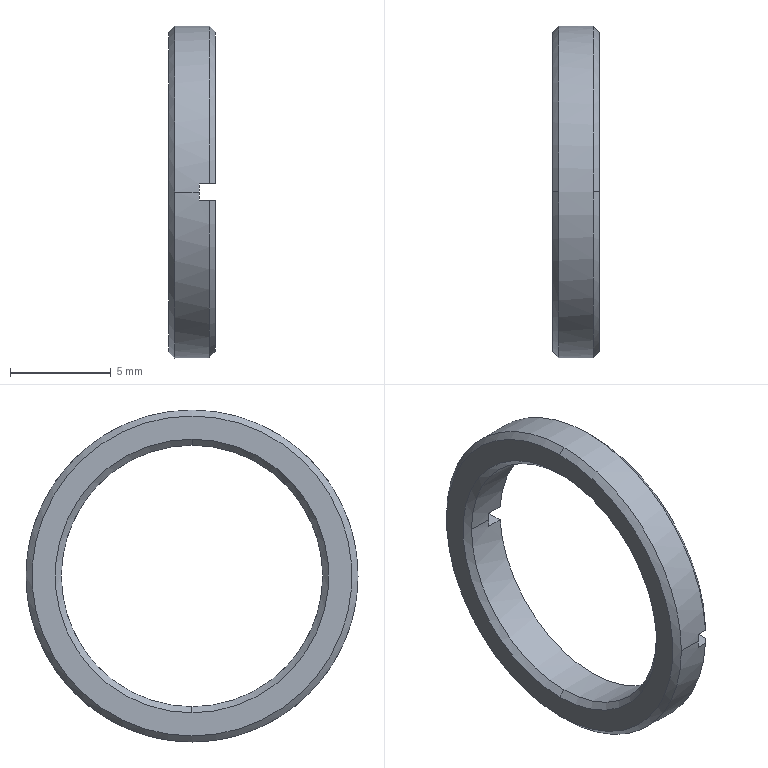Part | STEP file | pressure ring 2.stp.STEP-267.STEP | 1 solid | 20 faces | box 2.3 x 16.5 x 16.5 mm | volume 177.868 mm3 | plane 9 | cone 7 | cylinder 4 | commonest cylinder face diameters 13 x2 16.5 x2
STEP:
#1=CARTESIAN_POINT('',(421.126,0.,-8.25));
#2=VERTEX_POINT('',#1);
#3=CARTESIAN_POINT('',(421.126,8.25,0.));
#4=VERTEX_POINT('',#3);
#5=CARTESIAN_POINT('',(421.126,0.,0.));
#6=DIRECTION('',(1.,0.,0.));
#7=DIRECTION('',(0.,0.,1.));
#8=AXIS2_PLACEMENT_3D('',#5,#6,#7);
#9=CIRCLE('',#8,8.25);
#10=EDGE_CURVE('',#2,#4,#9,.T.);
#11=ORIENTED_EDGE('',*,*,#10,.T.);
#12=CARTESIAN_POINT('',(422.326,8.25,0.));
#13=VERTEX_POINT('',#12);
#14=CARTESIAN_POINT('',(0.,8.25,0.));
#15=DIRECTION('',(1.,0.,0.));
#16=VECTOR('',#15,1000.);
#17=LINE('',#14,#16);
#18=EDGE_CURVE('',#4,#13,#17,.T.);
#19=ORIENTED_EDGE('',*,*,#18,.T.);
#20=CARTESIAN_POINT('',(422.326,8.24,-0.4));
#21=VERTEX_POINT('',#20);
#22=CARTESIAN_POINT('',(422.326,0.,0.));
#23=DIRECTION('',(1.,0.,0.));
#24=DIRECTION('',(0.,0.,1.));
#25=AXIS2_PLACEMENT_3D('',#22,#23,#24);
#26=CIRCLE('',#25,8.25);
#27=EDGE_CURVE('',#21,#13,#26,.T.);
#28=ORIENTED_EDGE('',*,*,#27,.F.);
#29=CARTESIAN_POINT('',(422.826,8.24,-0.4));
#30=VERTEX_POINT('',#29);
#31=CARTESIAN_POINT('',(0.,8.24,-0.4));
#32=DIRECTION('',(1.,0.,0.));
#33=VECTOR('',#32,1000.);
#34=LINE('',#31,#33);
#35=EDGE_CURVE('',#21,#30,#34,.T.);
#36=ORIENTED_EDGE('',*,*,#35,.T.);
#37=CARTESIAN_POINT('',(422.826,-8.24,-0.4));
#38=VERTEX_POINT('',#37);
#39=CARTESIAN_POINT('',(422.826,0.,0.));
#40=DIRECTION('',(-1.,0.,0.));
#41=DIRECTION('',(0.,0.,-1.));
#42=AXIS2_PLACEMENT_3D('',#39,#40,#41);
#43=CIRCLE('',#42,8.25);
#44=EDGE_CURVE('',#30,#38,#43,.T.);
#45=ORIENTED_EDGE('',*,*,#44,.T.);
#46=CARTESIAN_POINT('',(422.326,-8.24,-0.4));
#47=VERTEX_POINT('',#46);
#48=CARTESIAN_POINT('',(0.,-8.24,-0.4));
#49=DIRECTION('',(-1.,0.,0.));
#50=VECTOR('',#49,1000.);
#51=LINE('',#48,#50);
#52=EDGE_CURVE('',#38,#47,#51,.T.);
#53=ORIENTED_EDGE('',*,*,#52,.T.);
#54=CARTESIAN_POINT('',(422.326,-8.25,0.));
#55=VERTEX_POINT('',#54);
#56=CARTESIAN_POINT('',(422.326,0.,0.));
#57=DIRECTION('',(1.,0.,0.));
#58=DIRECTION('',(0.,0.,1.));
#59=AXIS2_PLACEMENT_3D('',#56,#57,#58);
#60=CIRCLE('',#59,8.25);
#61=EDGE_CURVE('',#55,#47,#60,.T.);
#62=ORIENTED_EDGE('',*,*,#61,.F.);
#63=CARTESIAN_POINT('',(421.126,-8.25,0.));
#64=VERTEX_POINT('',#63);
#65=CARTESIAN_POINT('',(0.,-8.25,0.));
#66=DIRECTION('',(1.,0.,0.));
#67=VECTOR('',#66,1000.);
#68=LINE('',#65,#67);
#69=EDGE_CURVE('',#64,#55,#68,.T.);
#70=ORIENTED_EDGE('',*,*,#69,.F.);
#71=CARTESIAN_POINT('',(421.126,0.,0.));
#72=DIRECTION('',(1.,0.,0.));
#73=DIRECTION('',(0.,0.,1.));
#74=AXIS2_PLACEMENT_3D('',#71,#72,#73);
#75=CIRCLE('',#74,8.25);
#76=EDGE_CURVE('',#64,#2,#75,.T.);
#77=ORIENTED_EDGE('',*,*,#76,.T.);
#78=EDGE_LOOP('',(#11,#19,#28,#36,#45,#53,#62,#70,#77));
#79=FACE_OUTER_BOUND('',#78,.T.);
#80=CARTESIAN_POINT('',(0.,0.,0.));
#81=DIRECTION('',(1.,0.,0.));
#82=DIRECTION('',(0.,-1.,0.));
#83=AXIS2_PLACEMENT_3D('',#80,#81,#82);
#84=CYLINDRICAL_SURFACE('',#83,8.25);
#85=ADVANCED_FACE('',(#79),#84,.T.);
#86=CARTESIAN_POINT('',(421.126,0.,6.5));
#87=VERTEX_POINT('',#86);
#88=CARTESIAN_POINT('',(421.126,6.5,0.));
#89=VERTEX_POINT('',#88);
#90=CARTESIAN_POINT('',(421.126,0.,0.));
#91=DIRECTION('',(-1.,0.,0.));
#92=DIRECTION('',(0.,0.,1.));
#93=AXIS2_PLACEMENT_3D('',#90,#91,#92);
#94=CIRCLE('',#93,6.5);
#95=EDGE_CURVE('',#87,#89,#94,.T.);
#96=ORIENTED_EDGE('',*,*,#95,.T.);
#97=CARTESIAN_POINT('',(422.326,6.5,0.));
#98=VERTEX_POINT('',#97);
#99=CARTESIAN_POINT('',(0.,6.5,0.));
#100=DIRECTION('',(1.,0.,0.));
#101=VECTOR('',#100,1000.);
#102=LINE('',#99,#101);
#103=EDGE_CURVE('',#89,#98,#102,.T.);
#104=ORIENTED_EDGE('',*,*,#103,.T.);
#105=CARTESIAN_POINT('',(422.326,6.488,0.4));
#106=VERTEX_POINT('',#105);
#107=CARTESIAN_POINT('',(422.326,0.,0.));
#108=DIRECTION('',(-1.,0.,0.));
#109=DIRECTION('',(0.,0.,1.));
#110=AXIS2_PLACEMENT_3D('',#107,#108,#109);
#111=CIRCLE('',#110,6.5);
#112=EDGE_CURVE('',#106,#98,#111,.T.);
#113=ORIENTED_EDGE('',*,*,#112,.F.);
#114=CARTESIAN_POINT('',(423.126,6.488,0.4));
#115=VERTEX_POINT('',#114);
#116=CARTESIAN_POINT('',(0.,6.488,0.4));
#117=DIRECTION('',(1.,0.,0.));
#118=VECTOR('',#117,1000.);
#119=LINE('',#116,#118);
#120=EDGE_CURVE('',#106,#115,#119,.T.);
#121=ORIENTED_EDGE('',*,*,#120,.T.);
#122=CARTESIAN_POINT('',(423.126,-6.488,0.4));
#123=VERTEX_POINT('',#122);
#124=CARTESIAN_POINT('',(423.126,0.,0.));
#125=DIRECTION('',(1.,0.,0.));
#126=DIRECTION('',(0.,-1.,0.));
#127=AXIS2_PLACEMENT_3D('',#124,#125,#126);
#128=CIRCLE('',#127,6.5);
#129=EDGE_CURVE('',#115,#123,#128,.T.);
#130=ORIENTED_EDGE('',*,*,#129,.T.);
#131=CARTESIAN_POINT('',(422.326,-6.488,0.4));
#132=VERTEX_POINT('',#131);
#133=CARTESIAN_POINT('',(0.,-6.488,0.4));
#134=DIRECTION('',(-1.,0.,0.));
#135=VECTOR('',#134,1000.);
#136=LINE('',#133,#135);
#137=EDGE_CURVE('',#123,#132,#136,.T.);
#138=ORIENTED_EDGE('',*,*,#137,.T.);
#139=CARTESIAN_POINT('',(422.326,-6.5,0.));
#140=VERTEX_POINT('',#139);
#141=CARTESIAN_POINT('',(422.326,0.,0.));
#142=DIRECTION('',(-1.,0.,0.));
#143=DIRECTION('',(0.,0.,1.));
#144=AXIS2_PLACEMENT_3D('',#141,#142,#143);
#145=CIRCLE('',#144,6.5);
#146=EDGE_CURVE('',#140,#132,#145,.T.);
#147=ORIENTED_EDGE('',*,*,#146,.F.);
#148=CARTESIAN_POINT('',(421.126,-6.5,0.));
#149=VERTEX_POINT('',#148);
#150=CARTESIAN_POINT('',(0.,-6.5,0.));
#151=DIRECTION('',(1.,0.,0.));
#152=VECTOR('',#151,1000.);
#153=LINE('',#150,#152);
#154=EDGE_CURVE('',#149,#140,#153,.T.);
#155=ORIENTED_EDGE('',*,*,#154,.F.);
#156=CARTESIAN_POINT('',(421.126,0.,0.));
#157=DIRECTION('',(-1.,0.,0.));
#158=DIRECTION('',(0.,0.,1.));
#159=AXIS2_PLACEMENT_3D('',#156,#157,#158);
#160=CIRCLE('',#159,6.5);
#161=EDGE_CURVE('',#149,#87,#160,.T.);
#162=ORIENTED_EDGE('',*,*,#161,.T.);
#163=EDGE_LOOP('',(#96,#104,#113,#121,#130,#138,#147,#155,#162));
#164=FACE_OUTER_BOUND('',#163,.T.);
#165=CARTESIAN_POINT('',(0.,0.,0.));
#166=DIRECTION('',(1.,0.,0.));
#167=DIRECTION('',(0.,-1.,0.));
#168=AXIS2_PLACEMENT_3D('',#165,#166,#167);
#169=CYLINDRICAL_SURFACE('',#168,6.5);
#170=ADVANCED_FACE('',(#164),#169,.F.);
#171=CARTESIAN_POINT('',(421.126,0.,-6.5));
#172=VERTEX_POINT('',#171);
#173=CARTESIAN_POINT('',(421.126,0.,0.));
#174=DIRECTION('',(-1.,0.,0.));
#175=DIRECTION('',(0.,0.,1.));
#176=AXIS2_PLACEMENT_3D('',#173,#174,#175);
#177=CIRCLE('',#176,6.5);
#178=EDGE_CURVE('',#172,#149,#177,.T.);
#179=ORIENTED_EDGE('',*,*,#178,.F.);
#180=CARTESIAN_POINT('',(420.826,0.,-6.8));
#181=VERTEX_POINT('',#180);
#182=CARTESIAN_POINT('',(420.826,0.,-6.8));
#183=DIRECTION('',(-0.7071,0.,-0.7071));
#184=VECTOR('',#183,1000.);
#185=LINE('',#182,#184);
#186=EDGE_CURVE('',#172,#181,#185,.T.);
#187=ORIENTED_EDGE('',*,*,#186,.T.);
#188=CARTESIAN_POINT('',(420.826,0.,6.8));
#189=VERTEX_POINT('',#188);
#190=CARTESIAN_POINT('',(420.826,0.,0.));
#191=DIRECTION('',(1.,0.,0.));
#192=DIRECTION('',(0.,0.,1.));
#193=AXIS2_PLACEMENT_3D('',#190,#191,#192);
#194=CIRCLE('',#193,6.8);
#195=EDGE_CURVE('',#189,#181,#194,.T.);
#196=ORIENTED_EDGE('',*,*,#195,.F.);
#197=CARTESIAN_POINT('',(420.826,0.,6.8));
#198=DIRECTION('',(-0.7071,0.,0.7071));
#199=VECTOR('',#198,1000.);
#200=LINE('',#197,#199);
#201=EDGE_CURVE('',#87,#189,#200,.T.);
#202=ORIENTED_EDGE('',*,*,#201,.F.);
#203=ORIENTED_EDGE('',*,*,#161,.F.);
#204=EDGE_LOOP('',(#179,#187,#196,#202,#203));
#205=FACE_OUTER_BOUND('',#204,.T.);
#206=CARTESIAN_POINT('',(420.826,0.,0.));
#207=DIRECTION('',(-1.,0.,0.));
#208=DIRECTION('',(0.,0.,1.));
#209=AXIS2_PLACEMENT_3D('',#206,#207,#208);
#210=CONICAL_SURFACE('',#209,6.8,0.7854);
#211=ADVANCED_FACE('',(#205),#210,.F.);
#212=CARTESIAN_POINT('',(423.126,0.,7.95));
#213=VERTEX_POINT('',#212);
#214=CARTESIAN_POINT('',(423.126,-7.94,0.4));
#215=VERTEX_POINT('',#214);
#216=CARTESIAN_POINT('',(423.126,0.,0.));
#217=DIRECTION('',(1.,0.,0.));
#218=DIRECTION('',(0.,0.,-1.));
#219=AXIS2_PLACEMENT_3D('',#216,#217,#218);
#220=CIRCLE('',#219,7.95);
#221=EDGE_CURVE('',#213,#215,#220,.T.);
#222=ORIENTED_EDGE('',*,*,#221,.F.);
#223=CARTESIAN_POINT('',(422.826,0.,8.25));
#224=VERTEX_POINT('',#223);
#225=CARTESIAN_POINT('',(423.126,0.,7.95));
#226=DIRECTION('',(-0.7071,0.,0.7071));
#227=VECTOR('',#226,1000.);
#228=LINE('',#225,#227);
#229=EDGE_CURVE('',#213,#224,#228,.T.);
#230=ORIENTED_EDGE('',*,*,#229,.T.);
#231=CARTESIAN_POINT('',(422.826,-8.24,0.4));
#232=VERTEX_POINT('',#231);
#233=CARTESIAN_POINT('',(422.826,0.,0.));
#234=DIRECTION('',(-1.,0.,0.));
#235=DIRECTION('',(0.,0.,-1.));
#236=AXIS2_PLACEMENT_3D('',#233,#234,#235);
#237=CIRCLE('',#236,8.25);
#238=EDGE_CURVE('',#232,#224,#237,.T.);
#239=ORIENTED_EDGE('',*,*,#238,.F.);
#240=CARTESIAN_POINT('',(423.126,-7.94,0.4));
#241=CARTESIAN_POINT('',(423.026,-8.04,0.4));
#242=CARTESIAN_POINT('',(422.926,-8.14,0.4));
#243=CARTESIAN_POINT('',(422.826,-8.24,0.4));
#244=B_SPLINE_CURVE_WITH_KNOTS('',3,(#240,#241,#242,#243),.UNSPECIFIED.,.F.,.F.,(4,4),(0.,0.0004245),.UNSPECIFIED.);
#245=EDGE_CURVE('',#215,#232,#244,.T.);
#246=ORIENTED_EDGE('',*,*,#245,.F.);
#247=EDGE_LOOP('',(#222,#230,#239,#246));
#248=FACE_OUTER_BOUND('',#247,.T.);
#249=CARTESIAN_POINT('',(423.126,0.,0.));
#250=DIRECTION('',(-1.,0.,0.));
#251=DIRECTION('',(0.,0.,1.));
#252=AXIS2_PLACEMENT_3D('',#249,#250,#251);
#253=CONICAL_SURFACE('',#252,7.95,0.7854);
#254=ADVANCED_FACE('',(#248),#253,.T.);
#255=CARTESIAN_POINT('',(420.826,0.,7.95));
#256=VERTEX_POINT('',#255);
#257=CARTESIAN_POINT('',(420.826,0.,-7.95));
#258=VERTEX_POINT('',#257);
#259=CARTESIAN_POINT('',(420.826,0.,0.));
#260=DIRECTION('',(-1.,0.,0.));
#261=DIRECTION('',(0.,0.,1.));
#262=AXIS2_PLACEMENT_3D('',#259,#260,#261);
#263=CIRCLE('',#262,7.95);
#264=EDGE_CURVE('',#256,#258,#263,.T.);
#265=ORIENTED_EDGE('',*,*,#264,.F.);
#266=CARTESIAN_POINT('',(421.126,0.,8.25));
#267=VERTEX_POINT('',#266);
#268=CARTESIAN_POINT('',(421.126,0.,8.25));
#269=DIRECTION('',(0.7071,0.,0.7071));
#270=VECTOR('',#269,1000.);
#271=LINE('',#268,#270);
#272=EDGE_CURVE('',#256,#267,#271,.T.);
#273=ORIENTED_EDGE('',*,*,#272,.T.);
#274=CARTESIAN_POINT('',(421.126,0.,0.));
#275=DIRECTION('',(1.,0.,0.));
#276=DIRECTION('',(0.,0.,1.));
#277=AXIS2_PLACEMENT_3D('',#274,#275,#276);
#278=CIRCLE('',#277,8.25);
#279=EDGE_CURVE('',#4,#267,#278,.T.);
#280=ORIENTED_EDGE('',*,*,#279,.F.);
#281=ORIENTED_EDGE('',*,*,#10,.F.);
#282=CARTESIAN_POINT('',(421.126,0.,-8.25));
#283=DIRECTION('',(0.7071,0.,-0.7071));
#284=VECTOR('',#283,1000.);
#285=LINE('',#282,#284);
#286=EDGE_CURVE('',#258,#2,#285,.T.);
#287=ORIENTED_EDGE('',*,*,#286,.F.);
#288=EDGE_LOOP('',(#265,#273,#280,#281,#287));
#289=FACE_OUTER_BOUND('',#288,.T.);
#290=CARTESIAN_POINT('',(421.126,0.,0.));
#291=DIRECTION('',(1.,0.,0.));
#292=DIRECTION('',(0.,0.,-1.));
#293=AXIS2_PLACEMENT_3D('',#290,#291,#292);
#294=CONICAL_SURFACE('',#293,8.25,0.7854);
#295=ADVANCED_FACE('',(#289),#294,.T.);
#296=ORIENTED_EDGE('',*,*,#272,.F.);
#297=CARTESIAN_POINT('',(420.826,0.,0.));
#298=DIRECTION('',(-1.,0.,0.));
#299=DIRECTION('',(0.,0.,1.));
#300=AXIS2_PLACEMENT_3D('',#297,#298,#299);
#301=CIRCLE('',#300,7.95);
#302=EDGE_CURVE('',#258,#256,#301,.T.);
#303=ORIENTED_EDGE('',*,*,#302,.F.);
#304=ORIENTED_EDGE('',*,*,#286,.T.);
#305=ORIENTED_EDGE('',*,*,#76,.F.);
#306=CARTESIAN_POINT('',(421.126,0.,0.));
#307=DIRECTION('',(1.,0.,0.));
#308=DIRECTION('',(0.,0.,1.));
#309=AXIS2_PLACEMENT_3D('',#306,#307,#308);
#310=CIRCLE('',#309,8.25);
#311=EDGE_CURVE('',#267,#64,#310,.T.);
#312=ORIENTED_EDGE('',*,*,#311,.F.);
#313=EDGE_LOOP('',(#296,#303,#304,#305,#312));
#314=FACE_OUTER_BOUND('',#313,.T.);
#315=CARTESIAN_POINT('',(421.126,0.,0.));
#316=DIRECTION('',(1.,0.,0.));
#317=DIRECTION('',(0.,0.,-1.));
#318=AXIS2_PLACEMENT_3D('',#315,#316,#317);
#319=CONICAL_SURFACE('',#318,8.25,0.7854);
#320=ADVANCED_FACE('',(#314),#319,.T.);
#321=ORIENTED_EDGE('',*,*,#229,.F.);
#322=CARTESIAN_POINT('',(423.126,7.94,0.4));
#323=VERTEX_POINT('',#322);
#324=CARTESIAN_POINT('',(423.126,0.,0.));
#325=DIRECTION('',(1.,0.,0.));
#326=DIRECTION('',(0.,0.,-1.));
#327=AXIS2_PLACEMENT_3D('',#324,#325,#326);
#328=CIRCLE('',#327,7.95);
#329=EDGE_CURVE('',#323,#213,#328,.T.);
#330=ORIENTED_EDGE('',*,*,#329,.F.);
#331=CARTESIAN_POINT('',(422.826,8.24,0.4));
#332=VERTEX_POINT('',#331);
#333=CARTESIAN_POINT('',(422.826,8.24,0.4));
#334=CARTESIAN_POINT('',(422.926,8.14,0.4));
#335=CARTESIAN_POINT('',(423.026,8.04,0.4));
#336=CARTESIAN_POINT('',(423.126,7.94,0.4));
#337=B_SPLINE_CURVE_WITH_KNOTS('',3,(#333,#334,#335,#336),.UNSPECIFIED.,.F.,.F.,(4,4),(0.,0.0004245),.UNSPECIFIED.);
#338=EDGE_CURVE('',#332,#323,#337,.T.);
#339=ORIENTED_EDGE('',*,*,#338,.F.);
#340=CARTESIAN_POINT('',(422.826,0.,0.));
#341=DIRECTION('',(-1.,0.,0.));
#342=DIRECTION('',(0.,0.,-1.));
#343=AXIS2_PLACEMENT_3D('',#340,#341,#342);
#344=CIRCLE('',#343,8.25);
#345=EDGE_CURVE('',#224,#332,#344,.T.);
#346=ORIENTED_EDGE('',*,*,#345,.F.);
#347=EDGE_LOOP('',(#321,#330,#339,#346));
#348=FACE_OUTER_BOUND('',#347,.T.);
#349=CARTESIAN_POINT('',(423.126,0.,0.));
#350=DIRECTION('',(-1.,0.,0.));
#351=DIRECTION('',(0.,0.,1.));
#352=AXIS2_PLACEMENT_3D('',#349,#350,#351);
#353=CONICAL_SURFACE('',#352,7.95,0.7854);
#354=ADVANCED_FACE('',(#348),#353,.T.);
#355=CARTESIAN_POINT('',(423.126,10.,0.4));
#356=DIRECTION('',(0.,-1.,0.));
#357=VECTOR('',#356,1000.);
#358=LINE('',#355,#357);
#359=EDGE_CURVE('',#323,#115,#358,.T.);
#360=ORIENTED_EDGE('',*,*,#359,.F.);
#361=ORIENTED_EDGE('',*,*,#329,.T.);
#362=ORIENTED_EDGE('',*,*,#221,.T.);
#363=CARTESIAN_POINT('',(423.126,10.,0.4));
#364=DIRECTION('',(0.,-1.,0.));
#365=VECTOR('',#364,1000.);
#366=LINE('',#363,#365);
#367=EDGE_CURVE('',#123,#215,#366,.T.);
#368=ORIENTED_EDGE('',*,*,#367,.F.);
#369=ORIENTED_EDGE('',*,*,#129,.F.);
#370=EDGE_LOOP('',(#360,#361,#362,#368,#369));
#371=FACE_OUTER_BOUND('',#370,.T.);
#372=CARTESIAN_POINT('',(423.126,6.5,0.));
#373=DIRECTION('',(1.,0.,0.));
#374=DIRECTION('',(0.,1.,0.));
#375=AXIS2_PLACEMENT_3D('',#372,#373,#374);
#376=PLANE('',#375);
#377=ADVANCED_FACE('',(#371),#376,.T.);
#378=ORIENTED_EDGE('',*,*,#52,.F.);
#379=CARTESIAN_POINT('',(423.126,-7.94,-0.4));
#380=VERTEX_POINT('',#379);
#381=CARTESIAN_POINT('',(422.826,-8.24,-0.4));
#382=CARTESIAN_POINT('',(422.926,-8.14,-0.4));
#383=CARTESIAN_POINT('',(423.026,-8.04,-0.4));
#384=CARTESIAN_POINT('',(423.126,-7.94,-0.4));
#385=B_SPLINE_CURVE_WITH_KNOTS('',3,(#381,#382,#383,#384),.UNSPECIFIED.,.F.,.F.,(4,4),(0.,0.0004245),.UNSPECIFIED.);
#386=EDGE_CURVE('',#38,#380,#385,.T.);
#387=ORIENTED_EDGE('',*,*,#386,.T.);
#388=CARTESIAN_POINT('',(423.126,-6.488,-0.4));
#389=VERTEX_POINT('',#388);
#390=CARTESIAN_POINT('',(423.126,-10.,-0.4));
#391=DIRECTION('',(0.,1.,0.));
#392=VECTOR('',#391,1000.);
#393=LINE('',#390,#392);
#394=EDGE_CURVE('',#380,#389,#393,.T.);
#395=ORIENTED_EDGE('',*,*,#394,.T.);
#396=CARTESIAN_POINT('',(422.326,-6.488,-0.4));
#397=VERTEX_POINT('',#396);
#398=CARTESIAN_POINT('',(0.,-6.488,-0.4));
#399=DIRECTION('',(1.,0.,0.));
#400=VECTOR('',#399,1000.);
#401=LINE('',#398,#400);
#402=EDGE_CURVE('',#397,#389,#401,.T.);
#403=ORIENTED_EDGE('',*,*,#402,.F.);
#404=CARTESIAN_POINT('',(422.326,-10.,-0.4));
#405=DIRECTION('',(0.,1.,0.));
#406=VECTOR('',#405,1000.);
#407=LINE('',#404,#406);
#408=EDGE_CURVE('',#47,#397,#407,.T.);
#409=ORIENTED_EDGE('',*,*,#408,.F.);
#410=EDGE_LOOP('',(#378,#387,#395,#403,#409));
#411=FACE_OUTER_BOUND('',#410,.T.);
#412=CARTESIAN_POINT('',(422.326,-10.,-0.4));
#413=DIRECTION('',(0.,0.,1.));
#414=DIRECTION('',(0.,-1.,0.));
#415=AXIS2_PLACEMENT_3D('',#412,#413,#414);
#416=PLANE('',#415);
#417=ADVANCED_FACE('',(#411),#416,.T.);
#418=CARTESIAN_POINT('',(422.326,8.24,0.4));
#419=VERTEX_POINT('',#418);
#420=CARTESIAN_POINT('',(0.,8.24,0.4));
#421=DIRECTION('',(-1.,0.,0.));
#422=VECTOR('',#421,1000.);
#423=LINE('',#420,#422);
#424=EDGE_CURVE('',#332,#419,#423,.T.);
#425=ORIENTED_EDGE('',*,*,#424,.F.);
#426=ORIENTED_EDGE('',*,*,#338,.T.);
#427=ORIENTED_EDGE('',*,*,#359,.T.);
#428=ORIENTED_EDGE('',*,*,#120,.F.);
#429=CARTESIAN_POINT('',(422.326,10.,0.4));
#430=DIRECTION('',(0.,-1.,0.));
#431=VECTOR('',#430,1000.);
#432=LINE('',#429,#431);
#433=EDGE_CURVE('',#419,#106,#432,.T.);
#434=ORIENTED_EDGE('',*,*,#433,.F.);
#435=EDGE_LOOP('',(#425,#426,#427,#428,#434));
#436=FACE_OUTER_BOUND('',#435,.T.);
#437=CARTESIAN_POINT('',(422.326,10.,0.4));
#438=DIRECTION('',(0.,0.,-1.));
#439=DIRECTION('',(-1.,0.,0.));
#440=AXIS2_PLACEMENT_3D('',#437,#438,#439);
#441=PLANE('',#440);
#442=ADVANCED_FACE('',(#436),#441,.T.);
#443=CARTESIAN_POINT('',(423.126,6.488,-0.4));
#444=VERTEX_POINT('',#443);
#445=CARTESIAN_POINT('',(423.126,7.94,-0.4));
#446=VERTEX_POINT('',#445);
#447=CARTESIAN_POINT('',(423.126,-10.,-0.4));
#448=DIRECTION('',(0.,1.,0.));
#449=VECTOR('',#448,1000.);
#450=LINE('',#447,#449);
#451=EDGE_CURVE('',#444,#446,#450,.T.);
#452=ORIENTED_EDGE('',*,*,#451,.T.);
#453=CARTESIAN_POINT('',(423.126,7.94,-0.4));
#454=CARTESIAN_POINT('',(423.026,8.04,-0.4));
#455=CARTESIAN_POINT('',(422.926,8.14,-0.4));
#456=CARTESIAN_POINT('',(422.826,8.24,-0.4));
#457=B_SPLINE_CURVE_WITH_KNOTS('',3,(#453,#454,#455,#456),.UNSPECIFIED.,.F.,.F.,(4,4),(0.,0.0004245),.UNSPECIFIED.);
#458=EDGE_CURVE('',#446,#30,#457,.T.);
#459=ORIENTED_EDGE('',*,*,#458,.T.);
#460=ORIENTED_EDGE('',*,*,#35,.F.);
#461=CARTESIAN_POINT('',(422.326,6.488,-0.4));
#462=VERTEX_POINT('',#461);
#463=CARTESIAN_POINT('',(422.326,-10.,-0.4));
#464=DIRECTION('',(0.,1.,0.));
#465=VECTOR('',#464,1000.);
#466=LINE('',#463,#465);
#467=EDGE_CURVE('',#462,#21,#466,.T.);
#468=ORIENTED_EDGE('',*,*,#467,.F.);
#469=CARTESIAN_POINT('',(0.,6.488,-0.4));
#470=DIRECTION('',(-1.,0.,0.));
#471=VECTOR('',#470,1000.);
#472=LINE('',#469,#471);
#473=EDGE_CURVE('',#444,#462,#472,.T.);
#474=ORIENTED_EDGE('',*,*,#473,.F.);
#475=EDGE_LOOP('',(#452,#459,#460,#468,#474));
#476=FACE_OUTER_BOUND('',#475,.T.);
#477=CARTESIAN_POINT('',(422.326,-10.,-0.4));
#478=DIRECTION('',(0.,0.,1.));
#479=DIRECTION('',(0.,-1.,0.));
#480=AXIS2_PLACEMENT_3D('',#477,#478,#479);
#481=PLANE('',#480);
#482=ADVANCED_FACE('',(#476),#481,.T.);
#483=ORIENTED_EDGE('',*,*,#112,.T.);
#484=CARTESIAN_POINT('',(422.326,0.,0.));
#485=DIRECTION('',(-1.,0.,0.));
#486=DIRECTION('',(0.,0.,1.));
#487=AXIS2_PLACEMENT_3D('',#484,#485,#486);
#488=CIRCLE('',#487,6.5);
#489=EDGE_CURVE('',#98,#462,#488,.T.);
#490=ORIENTED_EDGE('',*,*,#489,.T.);
#491=ORIENTED_EDGE('',*,*,#467,.T.);
#492=ORIENTED_EDGE('',*,*,#27,.T.);
#493=CARTESIAN_POINT('',(422.326,0.,0.));
#494=DIRECTION('',(1.,0.,0.));
#495=DIRECTION('',(0.,0.,1.));
#496=AXIS2_PLACEMENT_3D('',#493,#494,#495);
#497=CIRCLE('',#496,8.25);
#498=EDGE_CURVE('',#13,#419,#497,.T.);
#499=ORIENTED_EDGE('',*,*,#498,.T.);
#500=ORIENTED_EDGE('',*,*,#433,.T.);
#501=EDGE_LOOP('',(#483,#490,#491,#492,#499,#500));
#502=FACE_OUTER_BOUND('',#501,.T.);
#503=CARTESIAN_POINT('',(422.326,10.,0.4));
#504=DIRECTION('',(-1.,0.,0.));
#505=DIRECTION('',(0.,0.,1.));
#506=AXIS2_PLACEMENT_3D('',#503,#504,#505);
#507=PLANE('',#506);
#508=ADVANCED_FACE('',(#502),#507,.F.);
#509=CARTESIAN_POINT('',(422.326,0.,0.));
#510=DIRECTION('',(-1.,0.,0.));
#511=DIRECTION('',(0.,0.,1.));
#512=AXIS2_PLACEMENT_3D('',#509,#510,#511);
#513=CIRCLE('',#512,6.5);
#514=EDGE_CURVE('',#397,#140,#513,.T.);
#515=ORIENTED_EDGE('',*,*,#514,.T.);
#516=ORIENTED_EDGE('',*,*,#146,.T.);
#517=CARTESIAN_POINT('',(422.326,-8.24,0.4));
#518=VERTEX_POINT('',#517);
#519=CARTESIAN_POINT('',(422.326,10.,0.4));
#520=DIRECTION('',(0.,-1.,0.));
#521=VECTOR('',#520,1000.);
#522=LINE('',#519,#521);
#523=EDGE_CURVE('',#132,#518,#522,.T.);
#524=ORIENTED_EDGE('',*,*,#523,.T.);
#525=CARTESIAN_POINT('',(422.326,0.,0.));
#526=DIRECTION('',(1.,0.,0.));
#527=DIRECTION('',(0.,0.,1.));
#528=AXIS2_PLACEMENT_3D('',#525,#526,#527);
#529=CIRCLE('',#528,8.25);
#530=EDGE_CURVE('',#518,#55,#529,.T.);
#531=ORIENTED_EDGE('',*,*,#530,.T.);
#532=ORIENTED_EDGE('',*,*,#61,.T.);
#533=ORIENTED_EDGE('',*,*,#408,.T.);
#534=EDGE_LOOP('',(#515,#516,#524,#531,#532,#533));
#535=FACE_OUTER_BOUND('',#534,.T.);
#536=CARTESIAN_POINT('',(422.326,10.,0.4));
#537=DIRECTION('',(-1.,0.,0.));
#538=DIRECTION('',(0.,0.,1.));
#539=AXIS2_PLACEMENT_3D('',#536,#537,#538);
#540=PLANE('',#539);
#541=ADVANCED_FACE('',(#535),#540,.F.);
#542=ORIENTED_EDGE('',*,*,#186,.F.);
#543=CARTESIAN_POINT('',(421.126,0.,0.));
#544=DIRECTION('',(-1.,0.,0.));
#545=DIRECTION('',(0.,0.,1.));
#546=AXIS2_PLACEMENT_3D('',#543,#544,#545);
#547=CIRCLE('',#546,6.5);
#548=EDGE_CURVE('',#89,#172,#547,.T.);
#549=ORIENTED_EDGE('',*,*,#548,.F.);
#550=ORIENTED_EDGE('',*,*,#95,.F.);
#551=ORIENTED_EDGE('',*,*,#201,.T.);
#552=CARTESIAN_POINT('',(420.826,0.,0.));
#553=DIRECTION('',(1.,0.,0.));
#554=DIRECTION('',(0.,0.,1.));
#555=AXIS2_PLACEMENT_3D('',#552,#553,#554);
#556=CIRCLE('',#555,6.8);
#557=EDGE_CURVE('',#181,#189,#556,.T.);
#558=ORIENTED_EDGE('',*,*,#557,.F.);
#559=EDGE_LOOP('',(#542,#549,#550,#551,#558));
#560=FACE_OUTER_BOUND('',#559,.T.);
#561=CARTESIAN_POINT('',(420.826,0.,0.));
#562=DIRECTION('',(-1.,0.,0.));
#563=DIRECTION('',(0.,0.,1.));
#564=AXIS2_PLACEMENT_3D('',#561,#562,#563);
#565=CONICAL_SURFACE('',#564,6.8,0.7854);
#566=ADVANCED_FACE('',(#560),#565,.F.);
#567=ORIENTED_EDGE('',*,*,#195,.T.);
#568=ORIENTED_EDGE('',*,*,#557,.T.);
#569=EDGE_LOOP('',(#567,#568));
#570=FACE_BOUND('',#569,.T.);
#571=ORIENTED_EDGE('',*,*,#302,.T.);
#572=ORIENTED_EDGE('',*,*,#264,.T.);
#573=EDGE_LOOP('',(#571,#572));
#574=FACE_OUTER_BOUND('',#573,.T.);
#575=CARTESIAN_POINT('',(420.826,8.25,0.));
#576=DIRECTION('',(-1.,0.,0.));
#577=DIRECTION('',(0.,0.,1.));
#578=AXIS2_PLACEMENT_3D('',#575,#576,#577);
#579=PLANE('',#578);
#580=ADVANCED_FACE('',(#570,#574),#579,.T.);
#581=ORIENTED_EDGE('',*,*,#103,.F.);
#582=ORIENTED_EDGE('',*,*,#548,.T.);
#583=ORIENTED_EDGE('',*,*,#178,.T.);
#584=ORIENTED_EDGE('',*,*,#154,.T.);
#585=ORIENTED_EDGE('',*,*,#514,.F.);
#586=ORIENTED_EDGE('',*,*,#402,.T.);
#587=CARTESIAN_POINT('',(423.126,0.,0.));
#588=DIRECTION('',(1.,0.,0.));
#589=DIRECTION('',(0.,-1.,0.));
#590=AXIS2_PLACEMENT_3D('',#587,#588,#589);
#591=CIRCLE('',#590,6.5);
#592=EDGE_CURVE('',#389,#444,#591,.T.);
#593=ORIENTED_EDGE('',*,*,#592,.T.);
#594=ORIENTED_EDGE('',*,*,#473,.T.);
#595=ORIENTED_EDGE('',*,*,#489,.F.);
#596=EDGE_LOOP('',(#581,#582,#583,#584,#585,#586,#593,#594,#595));
#597=FACE_OUTER_BOUND('',#596,.T.);
#598=CARTESIAN_POINT('',(0.,0.,0.));
#599=DIRECTION('',(1.,0.,0.));
#600=DIRECTION('',(0.,-1.,0.));
#601=AXIS2_PLACEMENT_3D('',#598,#599,#600);
#602=CYLINDRICAL_SURFACE('',#601,6.5);
#603=ADVANCED_FACE('',(#597),#602,.F.);
#604=ORIENTED_EDGE('',*,*,#394,.F.);
#605=CARTESIAN_POINT('',(423.126,0.,0.));
#606=DIRECTION('',(1.,0.,0.));
#607=DIRECTION('',(0.,0.,-1.));
#608=AXIS2_PLACEMENT_3D('',#605,#606,#607);
#609=CIRCLE('',#608,7.95);
#610=EDGE_CURVE('',#380,#446,#609,.T.);
#611=ORIENTED_EDGE('',*,*,#610,.T.);
#612=ORIENTED_EDGE('',*,*,#451,.F.);
#613=ORIENTED_EDGE('',*,*,#592,.F.);
#614=EDGE_LOOP('',(#604,#611,#612,#613));
#615=FACE_OUTER_BOUND('',#614,.T.);
#616=CARTESIAN_POINT('',(423.126,6.5,0.));
#617=DIRECTION('',(1.,0.,0.));
#618=DIRECTION('',(0.,1.,0.));
#619=AXIS2_PLACEMENT_3D('',#616,#617,#618);
#620=PLANE('',#619);
#621=ADVANCED_FACE('',(#615),#620,.T.);
#622=ORIENTED_EDGE('',*,*,#18,.F.);
#623=ORIENTED_EDGE('',*,*,#279,.T.);
#624=ORIENTED_EDGE('',*,*,#311,.T.);
#625=ORIENTED_EDGE('',*,*,#69,.T.);
#626=ORIENTED_EDGE('',*,*,#530,.F.);
#627=CARTESIAN_POINT('',(0.,-8.24,0.4));
#628=DIRECTION('',(1.,0.,0.));
#629=VECTOR('',#628,1000.);
#630=LINE('',#627,#629);
#631=EDGE_CURVE('',#518,#232,#630,.T.);
#632=ORIENTED_EDGE('',*,*,#631,.T.);
#633=ORIENTED_EDGE('',*,*,#238,.T.);
#634=ORIENTED_EDGE('',*,*,#345,.T.);
#635=ORIENTED_EDGE('',*,*,#424,.T.);
#636=ORIENTED_EDGE('',*,*,#498,.F.);
#637=EDGE_LOOP('',(#622,#623,#624,#625,#626,#632,#633,#634,#635,#636));
#638=FACE_OUTER_BOUND('',#637,.T.);
#639=CARTESIAN_POINT('',(0.,0.,0.));
#640=DIRECTION('',(1.,0.,0.));
#641=DIRECTION('',(0.,-1.,0.));
#642=AXIS2_PLACEMENT_3D('',#639,#640,#641);
#643=CYLINDRICAL_SURFACE('',#642,8.25);
#644=ADVANCED_FACE('',(#638),#643,.T.);
#645=ORIENTED_EDGE('',*,*,#367,.T.);
#646=ORIENTED_EDGE('',*,*,#245,.T.);
#647=ORIENTED_EDGE('',*,*,#631,.F.);
#648=ORIENTED_EDGE('',*,*,#523,.F.);
#649=ORIENTED_EDGE('',*,*,#137,.F.);
#650=EDGE_LOOP('',(#645,#646,#647,#648,#649));
#651=FACE_OUTER_BOUND('',#650,.T.);
#652=CARTESIAN_POINT('',(422.326,10.,0.4));
#653=DIRECTION('',(0.,0.,-1.));
#654=DIRECTION('',(-1.,0.,0.));
#655=AXIS2_PLACEMENT_3D('',#652,#653,#654);
#656=PLANE('',#655);
#657=ADVANCED_FACE('',(#651),#656,.T.);
#658=ORIENTED_EDGE('',*,*,#386,.F.);
#659=ORIENTED_EDGE('',*,*,#44,.F.);
#660=ORIENTED_EDGE('',*,*,#458,.F.);
#661=ORIENTED_EDGE('',*,*,#610,.F.);
#662=EDGE_LOOP('',(#658,#659,#660,#661));
#663=FACE_OUTER_BOUND('',#662,.T.);
#664=CARTESIAN_POINT('',(423.126,0.,0.));
#665=DIRECTION('',(-1.,0.,0.));
#666=DIRECTION('',(0.,0.,1.));
#667=AXIS2_PLACEMENT_3D('',#664,#665,#666);
#668=CONICAL_SURFACE('',#667,7.95,0.7854);
#669=ADVANCED_FACE('',(#663),#668,.T.);
#670=CLOSED_SHELL('',(#85,#170,#211,#254,#295,#320,#354,#377,#417,#442,#482,#508,#541,#566,#580,#603,#621,#644,#657,#669));
#671=MANIFOLD_SOLID_BREP('',#670);
#672=CARTESIAN_POINT('',(0.,0.,0.));
#673=DIRECTION('',(0.,0.,1.));
#674=DIRECTION('',(1.,0.,0.));
#675=AXIS2_PLACEMENT_3D('',#672,#673,#674);
#676=(LENGTH_UNIT()NAMED_UNIT(*)SI_UNIT(.MILLI.,.METRE.));
#677=UNCERTAINTY_MEASURE_WITH_UNIT(LENGTH_MEASURE(0.00001),#676,'','');
#678=(NAMED_UNIT(*)PLANE_ANGLE_UNIT()SI_UNIT($,.RADIAN.));
#679=(NAMED_UNIT(*)SI_UNIT($,.STERADIAN.)SOLID_ANGLE_UNIT());
#680=(GEOMETRIC_REPRESENTATION_CONTEXT(3)GLOBAL_UNCERTAINTY_ASSIGNED_CONTEXT((#677))GLOBAL_UNIT_ASSIGNED_CONTEXT((#676,#678,#679))REPRESENTATION_CONTEXT('',''));
#681=ADVANCED_BREP_SHAPE_REPRESENTATION('',(#671,#675),#680);